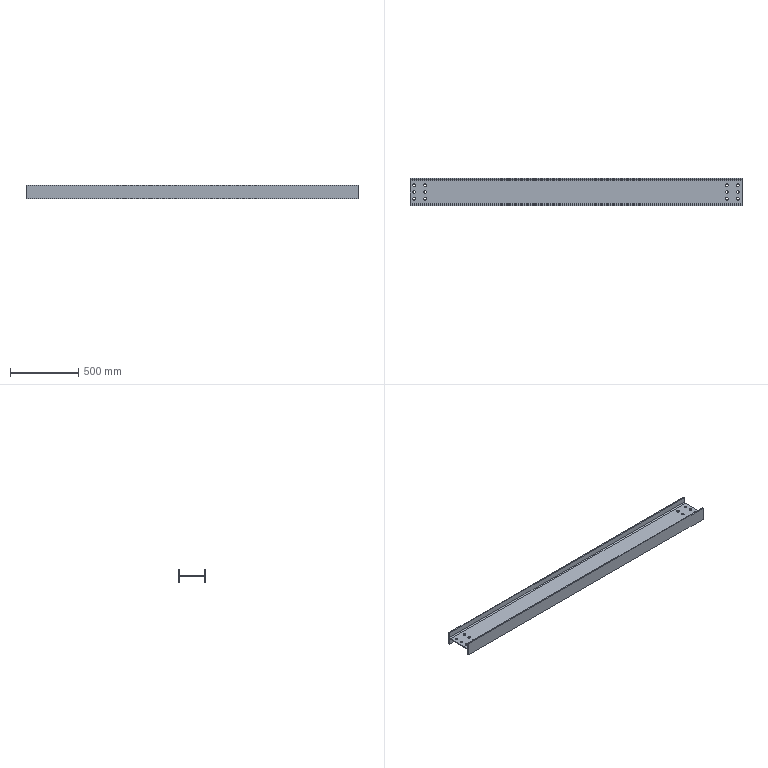Part | STEP file | 电柜主梁4主体_Default<As Machined> | 1 solid | 42 faces | box 2430 x 200 x 100 mm | volume 6461947 mm3 | cylinder 28 | plane 14 | commonest cylinder face diameters 19 x24 16 x4